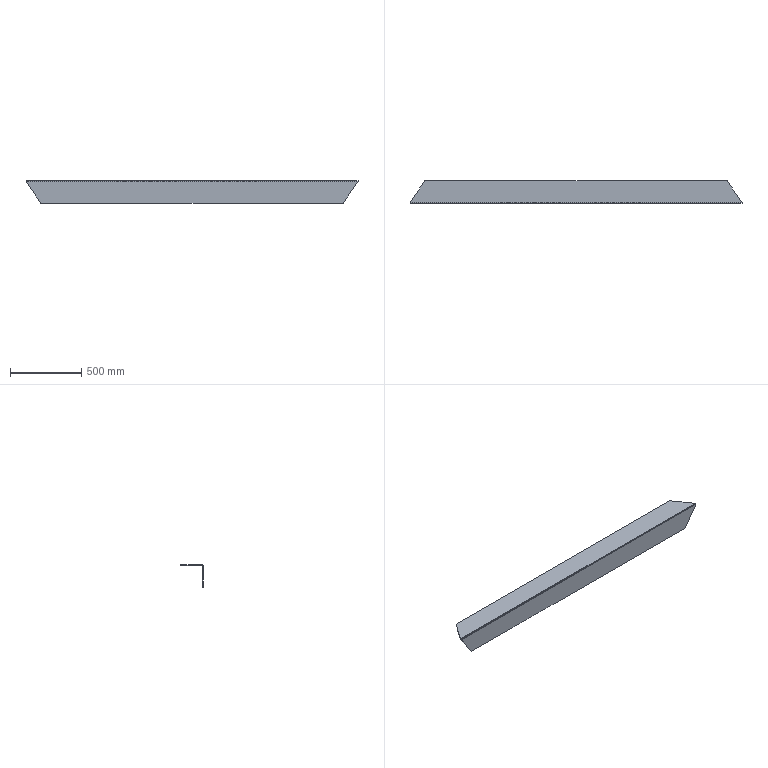Part | SolidWorks | 2 solids | 12 faces | box 2328 x 156 x 156 mm | volume 4001344 mm3 | plane 12